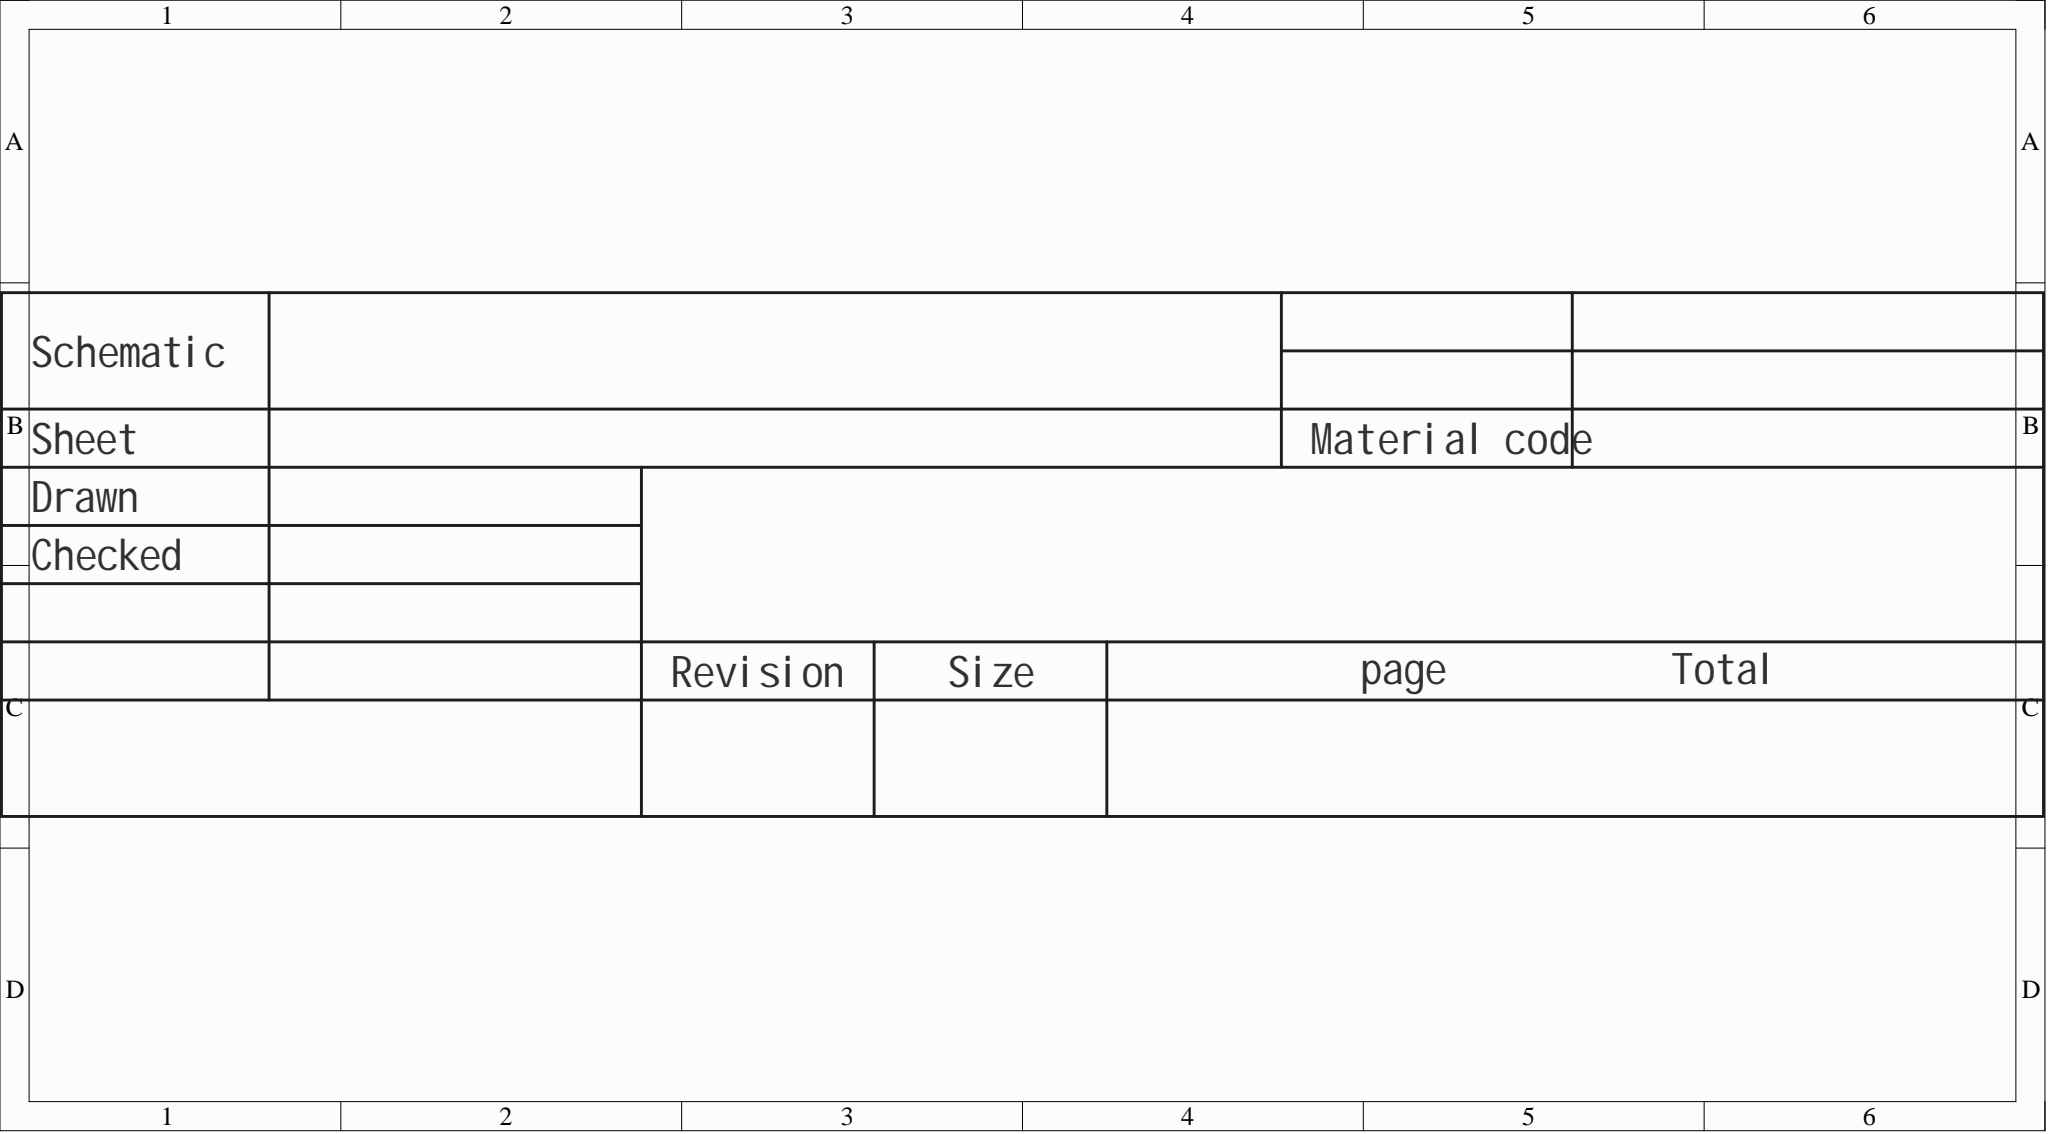Circuit board | Altium Designer | 30 parts | 36 nets
Bill of materials:
Comment,Description,Designator,Footprint,LibRef,Quantity
"buzzer-12X9","","BUZZER1","BUZ-TH_BD12.0-P7.60-D0.6-FD","buzzer-12X9","1"
"10uf","","C1","C0805","CAP_0805","1"
"30pf","","C2, C3","C0805","CAP_0805","2"
"","","H1","HDR-TH_9P-P2.54-V-F-1","HDR-F_2.54_1x9P","1"
"","","H2","HDR-TH_6P-P2.54-V-M-1","HDR-M_2.54_1x6P","1"
"","","H3, H4","HDR-TH_4P-P2.54-V-M","HDR-M_2.54_1x4P","2"
"","","H5","HDR-TH_2P-P2.54-V-M-1","HDR-M_2.54_1x2P","1"
"LMB162ADC","16x2 character LCD module","LCD1","LCD1602","LMB162ADC","1"
"","","LEDG1, LEDG2, LEDR1","LED_0805","LED_0805-R","3"
"2N3906S-RTK/PS","","Q1","SOT-23-3_L2.9-W1.3-P1.90-LS2.4-TR","2N3906S-RTK/PS","1"
"10K","","R1, R2","R0805","Res_0805","2"
"1K","","R3","R0805","Res_0805","1"
"220","","R4, R5, R7","R0805","Res_0805","3"
"2.2K","","R6","R0805","Res_0805","1"
"Tact switch 3*6*2.5","","SW1, SW2, SW3, SW4","SW-SMD_L6.0-W3.6-LS8.0","轻触按键3*6*2.5","4"
"DSWB04LHGET","Type:Flat toggle, raised;Circuit:SPST;Positions:4;Service life:-;Color:Red;","SW5","SW-TH_DSWB04LHGET","DSWB04LHGET","1"
"STC89C516RD+40I-PDIP40","CPU core:51 series;Program memory capacity:61KB;Total RAM:1.25KB;GPIO port count:35;Operating voltage range:3.5V~5.5V;Max CPU frequency:-;Program memory type:FLASH;","U1","DIP-40_L52.3-W13.9-P2.54-LS15.2-BL","STC89C516RD+40I-PDIP40","1"
"11.059MHz","Frequency:12MHz;Frequency tolerance at room temp:±30ppm;Load capacitance:-;Frequency stability (full temp):±50ppm;","U2","HC-49US_L11.0-W4.6-P4.88","ECS-120-S-4","1"
"SN74LS126ADR2","","U5","SOIC-14_L8.7-W3.9-P1.27-LS6.0-BL","SN74LS126ADR2","1"
"DM74LS125ASJ","Supply voltage:4.75V~5.25V;Element count:4;Bits per element:1;Sink current (IOL):24mA;Source current (IOH):2.6mA;","U6","SOP-14_L10.2-W5.3-P1.27-LS7.8-BL","DM74LS125ASJ","1"
Netlist (Protel format):
[
BUZZER1
BUZ-TH_BD12.0-P7.60-D0.6-FD
buzzer-12X9



]
[
C1
C0805
10uf



]
[
C2
C0805
30pf



]
[
C3
C0805
30pf



]
[
H1
HDR-TH_9P-P2.54-V-F-1




]
[
H2
HDR-TH_6P-P2.54-V-M-1




]
[
H3
HDR-TH_4P-P2.54-V-M




]
[
H4
HDR-TH_4P-P2.54-V-M




]
[
H5
HDR-TH_2P-P2.54-V-M-1




]
[
LCD1
LCD1602
LMB162ADC



]
[
LEDG1
LED_0805




]
[
LEDG2
LED_0805




]
[
LEDR1
LED_0805




]
[
Q1
SOT-23-3_L2.9-W1.3-P1.90-LS2.4-TR
2N3906S-RTK/PS



]
[
R1
R0805
10K



]
[
R2
R0805
10K



]
[
R3
R0805
1K



]
[
R4
R0805
220



]
[
R5
R0805
220



]
[
R6
R0805
2.2K



]
[
R7
R0805
220



]
[
SW1
SW-SMD_L6.0-W3.6-LS8.0
Tact switch 3*6*2.5



]
[
SW2
SW-SMD_L6.0-W3.6-LS8.0
Tact switch 3*6*2.5



]
[
SW3
SW-SMD_L6.0-W3.6-LS8.0
Tact switch 3*6*2.5



]
[
SW4
SW-SMD_L6.0-W3.6-LS8.0
Tact switch 3*6*2.5



]
[
SW5
SW-TH_DSWB04LHGET
DSWB04LHGET



]
[
U1
DIP-40_L52.3-W13.9-P2.54-LS15.2-BL
STC89C516RD+40I-PDIP40



]
[
U2
HC-49US_L11.0-W4.6-P4.88
11.0592MHz



]
[
U5
SOIC-14_L8.7-W3.9-P1.27-LS6.0-BL
SN74LS126ADR2



]
[
U6
SOP-14_L10.2-W5.3-P1.27-LS7.8-BL
DM74LS125ASJ



]
(
VCC
BUZZER1-2
C1-2
H1-1
H2-2
H3-3
H4-4
H5-2
LCD1-2
LCD1-15
R2-2
R4-2
R5-2
R7-2
SW1-2
U1-40
U5-14
U6-14
)
(
TX2
H3-2
U6-5
)
(
TX1
H2-4
U5-5
)
(
TX0
H4-2
SW5-3
SW5-4
U1-11
)
(
TX
SW5-7
SW5-8
U5-2
U6-2
)
(
RX2
H3-1
U6-3
)
(
RX1
H2-5
U5-3
)
(
RX0
H4-1
SW5-1
SW5-2
U1-10
)
(
RX
SW5-5
SW5-6
U5-6
U6-6
)
(
RS
LCD1-4
U1-24
)
(
NetU1_14
U1-14
U5-1
U5-4
U6-1
U6-4
)
(
NetSW4_1
SW4-1
U1-17
)
(
NetSW3_1
SW3-1
U1-28
)
(
NetSW2_1
SW2-1
U1-27
)
(
NetR6_1
R6-1
U1-26
)
(
NetQ1_2
Q1-2
R6-2
)
(
NetLEDR1_2
LEDR1-2
R4-1
)
(
NetLEDR1_1
LEDR1-1
U1-23
)
(
NetLEDG2_2
LEDG2-2
R7-1
)
(
NetLEDG1_2
LEDG1-2
R5-1
)
(
NetLEDG1_1
LEDG1-1
U1-21
)
(
NetLCD1_3
LCD1-3
R2-1
R3-2
)
(
NetH1_9
H1-9
LCD1-14
U1-32
)
(
NetH1_8
H1-8
LCD1-13
U1-33
)
(
NetH1_7
H1-7
LCD1-12
U1-34
)
(
NetH1_6
H1-6
LCD1-11
U1-35
)
(
NetH1_5
H1-5
LCD1-10
U1-36
)
(
NetH1_4
H1-4
LCD1-9
U1-37
)
(
NetH1_3
H1-3
LCD1-8
U1-38
)
(
NetH1_2
H1-2
LCD1-7
U1-39
)
(
NetC3_2
C3-2
U1-19
U2-2
)
(
NetC2_2
C2-2
U1-18
U2-1
)
(
NetC1_1
C1-1
R1-1
SW1-1
U1-9
)
(
NetBUZZER1_1
BUZZER1-1
Q1-1
)
(
GND
C2-1
C3-1
H2-3
H3-4
H4-3
H5-1
LCD1-1
LCD1-5
LCD1-16
LEDG2-1
Q1-3
R1-2
R3-1
SW2-2
SW3-2
SW4-2
U1-20
U5-7
U6-7
)
(
EN
LCD1-6
U1-25
)